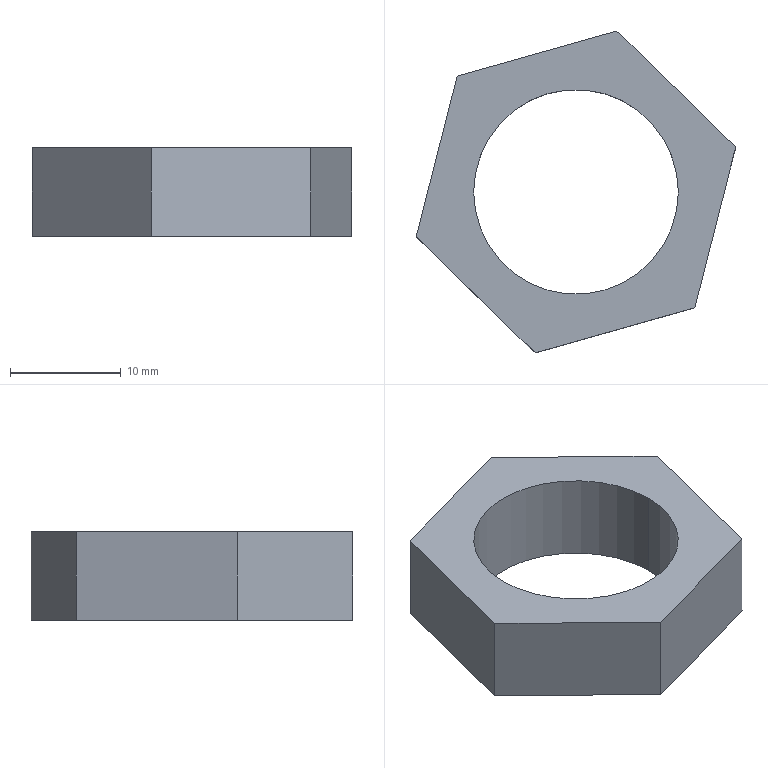Part | STEP file | 1 solid | 10 faces | box 28.896 x 29.097 x 8 mm | volume 2533 mm3 | plane 8 | cylinder 2 | commonest cylinder face diameters 18.5 x2
STEP:
#1=CARTESIAN_POINT('',(0.,0.,0.));
#2=DIRECTION('',(0.,0.,1.));
#3=DIRECTION('',(1.,0.,0.));
#4=AXIS2_PLACEMENT_3D('',#1,#2,#3);
#5=CARTESIAN_POINT('',(9.25,0.,0.));
#6=VERTEX_POINT('',#5);
#7=CARTESIAN_POINT('',(9.25,0.,8.));
#8=VERTEX_POINT('',#7);
#9=CARTESIAN_POINT('',(9.25,0.,0.));
#10=DIRECTION('',(0.,0.,1.));
#11=VECTOR('',#10,1.);
#12=LINE('',#9,#11);
#13=CARTESIAN_POINT('',(0.,0.,0.));
#14=DIRECTION('',(0.,0.,1.));
#15=DIRECTION('',(1.,0.,0.));
#16=AXIS2_PLACEMENT_3D('',#13,#14,#15);
#17=CYLINDRICAL_SURFACE('',#16,9.25);
#18=CARTESIAN_POINT('',(6.283,0.));
#19=DIRECTION('',(0.,1.));
#20=VECTOR('',#19,1.);
#21=LINE('',#18,#20);
#22=(GEOMETRIC_REPRESENTATION_CONTEXT(2)PARAMETRIC_REPRESENTATION_CONTEXT()REPRESENTATION_CONTEXT('',''));
#23=DEFINITIONAL_REPRESENTATION('',(#21),#22);
#24=PCURVE('',#17,#23);
#25=CARTESIAN_POINT('',(0.,0.,0.));
#26=DIRECTION('',(0.,0.,1.));
#27=DIRECTION('',(1.,0.,0.));
#28=AXIS2_PLACEMENT_3D('',#25,#26,#27);
#29=CYLINDRICAL_SURFACE('',#28,9.25);
#30=CARTESIAN_POINT('',(0.,0.));
#31=DIRECTION('',(0.,1.));
#32=VECTOR('',#31,1.);
#33=LINE('',#30,#32);
#34=(GEOMETRIC_REPRESENTATION_CONTEXT(2)PARAMETRIC_REPRESENTATION_CONTEXT()REPRESENTATION_CONTEXT('',''));
#35=DEFINITIONAL_REPRESENTATION('',(#33),#34);
#36=PCURVE('',#29,#35);
#37=SURFACE_CURVE('',#12,(#24,#36),.PCURVE_S1.);
#38=EDGE_CURVE('',#6,#8,#37,.T.);
#39=ORIENTED_EDGE('',*,*,#38,.T.);
#40=CARTESIAN_POINT('',(-9.25,0.,8.));
#41=VERTEX_POINT('',#40);
#42=CARTESIAN_POINT('',(0.,0.,8.));
#43=DIRECTION('',(0.,0.,1.));
#44=DIRECTION('',(1.,0.,0.));
#45=AXIS2_PLACEMENT_3D('',#42,#43,#44);
#46=CIRCLE('',#45,9.25);
#47=CARTESIAN_POINT('',(0.,8.));
#48=DIRECTION('',(1.,0.));
#49=VECTOR('',#48,1.);
#50=LINE('',#47,#49);
#51=(GEOMETRIC_REPRESENTATION_CONTEXT(2)PARAMETRIC_REPRESENTATION_CONTEXT()REPRESENTATION_CONTEXT('',''));
#52=DEFINITIONAL_REPRESENTATION('',(#50),#51);
#53=PCURVE('',#17,#52);
#54=CARTESIAN_POINT('',(-14.622,-14.723,8.));
#55=DIRECTION('',(0.,0.,1.));
#56=DIRECTION('',(1.,0.,0.));
#57=AXIS2_PLACEMENT_3D('',#54,#55,#56);
#58=PLANE('',#57);
#59=CARTESIAN_POINT('',(14.622,14.723));
#60=DIRECTION('',(1.,0.));
#61=AXIS2_PLACEMENT_2D('',#59,#60);
#62=CIRCLE('',#61,9.25);
#63=(GEOMETRIC_REPRESENTATION_CONTEXT(2)PARAMETRIC_REPRESENTATION_CONTEXT()REPRESENTATION_CONTEXT('',''));
#64=DEFINITIONAL_REPRESENTATION('',(#62),#63);
#65=PCURVE('',#58,#64);
#66=SURFACE_CURVE('',#46,(#53,#65),.PCURVE_S1.);
#67=EDGE_CURVE('',#41,#8,#66,.T.);
#68=ORIENTED_EDGE('',*,*,#67,.F.);
#69=CARTESIAN_POINT('',(-9.25,0.,0.));
#70=VERTEX_POINT('',#69);
#71=CARTESIAN_POINT('',(-9.25,0.,0.));
#72=DIRECTION('',(0.,0.,1.));
#73=VECTOR('',#72,1.);
#74=LINE('',#71,#73);
#75=CARTESIAN_POINT('',(3.142,0.));
#76=DIRECTION('',(0.,1.));
#77=VECTOR('',#76,1.);
#78=LINE('',#75,#77);
#79=(GEOMETRIC_REPRESENTATION_CONTEXT(2)PARAMETRIC_REPRESENTATION_CONTEXT()REPRESENTATION_CONTEXT('',''));
#80=DEFINITIONAL_REPRESENTATION('',(#78),#79);
#81=PCURVE('',#17,#80);
#82=CARTESIAN_POINT('',(3.142,0.));
#83=DIRECTION('',(0.,1.));
#84=VECTOR('',#83,1.);
#85=LINE('',#82,#84);
#86=(GEOMETRIC_REPRESENTATION_CONTEXT(2)PARAMETRIC_REPRESENTATION_CONTEXT()REPRESENTATION_CONTEXT('',''));
#87=DEFINITIONAL_REPRESENTATION('',(#85),#86);
#88=PCURVE('',#29,#87);
#89=SURFACE_CURVE('',#74,(#81,#88),.PCURVE_S1.);
#90=EDGE_CURVE('',#70,#41,#89,.T.);
#91=ORIENTED_EDGE('',*,*,#90,.F.);
#92=CARTESIAN_POINT('',(0.,0.,0.));
#93=DIRECTION('',(0.,0.,-1.));
#94=DIRECTION('',(1.,0.,0.));
#95=AXIS2_PLACEMENT_3D('',#92,#93,#94);
#96=CIRCLE('',#95,9.25);
#97=CARTESIAN_POINT('',(6.283,0.));
#98=DIRECTION('',(-1.,0.));
#99=VECTOR('',#98,1.);
#100=LINE('',#97,#99);
#101=(GEOMETRIC_REPRESENTATION_CONTEXT(2)PARAMETRIC_REPRESENTATION_CONTEXT()REPRESENTATION_CONTEXT('',''));
#102=DEFINITIONAL_REPRESENTATION('',(#100),#101);
#103=PCURVE('',#17,#102);
#104=CARTESIAN_POINT('',(-14.622,-14.723,0.));
#105=DIRECTION('',(0.,0.,1.));
#106=DIRECTION('',(1.,0.,0.));
#107=AXIS2_PLACEMENT_3D('',#104,#105,#106);
#108=PLANE('',#107);
#109=CARTESIAN_POINT('',(23.872,14.723));
#110=CARTESIAN_POINT('',(23.872,-1.298));
#111=CARTESIAN_POINT('',(9.997,6.712));
#112=CARTESIAN_POINT('',(-3.878,14.723));
#113=CARTESIAN_POINT('',(9.997,22.734));
#114=CARTESIAN_POINT('',(23.872,30.745));
#115=CARTESIAN_POINT('',(23.872,14.723));
#116=(BOUNDED_CURVE()B_SPLINE_CURVE(2,(#109,#110,#111,#112,#113,#114,#115),.UNSPECIFIED.,.T.,.F.)B_SPLINE_CURVE_WITH_KNOTS((1,2,2,2,2,1),(-2.094,0.,2.094,4.189,6.283,8.378),.UNSPECIFIED.)CURVE()GEOMETRIC_REPRESENTATION_ITEM()RATIONAL_B_SPLINE_CURVE((1.,0.5,1.,0.5,1.,0.5,1.))REPRESENTATION_ITEM(''));
#117=(GEOMETRIC_REPRESENTATION_CONTEXT(2)PARAMETRIC_REPRESENTATION_CONTEXT()REPRESENTATION_CONTEXT('',''));
#118=DEFINITIONAL_REPRESENTATION('',(#116),#117);
#119=PCURVE('',#108,#118);
#120=SURFACE_CURVE('',#96,(#103,#119),.PCURVE_S1.);
#121=EDGE_CURVE('',#6,#70,#120,.T.);
#122=ORIENTED_EDGE('',*,*,#121,.F.);
#123=EDGE_LOOP('',(#39,#68,#91,#122));
#124=FACE_BOUND('',#123,.F.);
#125=ADVANCED_FACE('',(#124),#17,.F.);
#126=CARTESIAN_POINT('',(0.,0.,8.));
#127=DIRECTION('',(0.,0.,1.));
#128=DIRECTION('',(1.,0.,0.));
#129=AXIS2_PLACEMENT_3D('',#126,#127,#128);
#130=CIRCLE('',#129,9.25);
#131=CARTESIAN_POINT('',(0.,8.));
#132=DIRECTION('',(1.,0.));
#133=VECTOR('',#132,1.);
#134=LINE('',#131,#133);
#135=(GEOMETRIC_REPRESENTATION_CONTEXT(2)PARAMETRIC_REPRESENTATION_CONTEXT()REPRESENTATION_CONTEXT('',''));
#136=DEFINITIONAL_REPRESENTATION('',(#134),#135);
#137=PCURVE('',#29,#136);
#138=CARTESIAN_POINT('',(14.622,14.723));
#139=DIRECTION('',(1.,0.));
#140=AXIS2_PLACEMENT_2D('',#138,#139);
#141=CIRCLE('',#140,9.25);
#142=(GEOMETRIC_REPRESENTATION_CONTEXT(2)PARAMETRIC_REPRESENTATION_CONTEXT()REPRESENTATION_CONTEXT('',''));
#143=DEFINITIONAL_REPRESENTATION('',(#141),#142);
#144=PCURVE('',#58,#143);
#145=SURFACE_CURVE('',#130,(#137,#144),.PCURVE_S1.);
#146=EDGE_CURVE('',#8,#41,#145,.T.);
#147=ORIENTED_EDGE('',*,*,#146,.F.);
#148=ORIENTED_EDGE('',*,*,#38,.F.);
#149=CARTESIAN_POINT('',(0.,0.,0.));
#150=DIRECTION('',(0.,0.,-1.));
#151=DIRECTION('',(1.,0.,0.));
#152=AXIS2_PLACEMENT_3D('',#149,#150,#151);
#153=CIRCLE('',#152,9.25);
#154=CARTESIAN_POINT('',(6.283,0.));
#155=DIRECTION('',(-1.,0.));
#156=VECTOR('',#155,1.);
#157=LINE('',#154,#156);
#158=(GEOMETRIC_REPRESENTATION_CONTEXT(2)PARAMETRIC_REPRESENTATION_CONTEXT()REPRESENTATION_CONTEXT('',''));
#159=DEFINITIONAL_REPRESENTATION('',(#157),#158);
#160=PCURVE('',#29,#159);
#161=CARTESIAN_POINT('',(23.872,14.723));
#162=CARTESIAN_POINT('',(23.872,-1.298));
#163=CARTESIAN_POINT('',(9.997,6.712));
#164=CARTESIAN_POINT('',(-3.878,14.723));
#165=CARTESIAN_POINT('',(9.997,22.734));
#166=CARTESIAN_POINT('',(23.872,30.745));
#167=CARTESIAN_POINT('',(23.872,14.723));
#168=(BOUNDED_CURVE()B_SPLINE_CURVE(2,(#161,#162,#163,#164,#165,#166,#167),.UNSPECIFIED.,.T.,.F.)B_SPLINE_CURVE_WITH_KNOTS((1,2,2,2,2,1),(-2.094,0.,2.094,4.189,6.283,8.378),.UNSPECIFIED.)CURVE()GEOMETRIC_REPRESENTATION_ITEM()RATIONAL_B_SPLINE_CURVE((1.,0.5,1.,0.5,1.,0.5,1.))REPRESENTATION_ITEM(''));
#169=(GEOMETRIC_REPRESENTATION_CONTEXT(2)PARAMETRIC_REPRESENTATION_CONTEXT()REPRESENTATION_CONTEXT('',''));
#170=DEFINITIONAL_REPRESENTATION('',(#168),#169);
#171=PCURVE('',#108,#170);
#172=SURFACE_CURVE('',#153,(#160,#171),.PCURVE_S1.);
#173=EDGE_CURVE('',#70,#6,#172,.T.);
#174=ORIENTED_EDGE('',*,*,#173,.F.);
#175=ORIENTED_EDGE('',*,*,#90,.T.);
#176=EDGE_LOOP('',(#147,#148,#174,#175));
#177=FACE_BOUND('',#176,.F.);
#178=ADVANCED_FACE('',(#177),#29,.F.);
#179=ORIENTED_EDGE('',*,*,#146,.F.);
#180=ORIENTED_EDGE('',*,*,#67,.F.);
#181=EDGE_LOOP('',(#179,#180));
#182=FACE_BOUND('',#181,.T.);
#183=CARTESIAN_POINT('',(-10.751,10.476,8.));
#184=VERTEX_POINT('',#183);
#185=CARTESIAN_POINT('',(-14.448,-4.072,8.));
#186=VERTEX_POINT('',#185);
#187=CARTESIAN_POINT('',(-10.751,10.476,8.));
#188=DIRECTION('',(-0.2463,-0.9692,0.));
#189=VECTOR('',#188,1.);
#190=LINE('',#187,#189);
#191=CARTESIAN_POINT('',(3.871,25.2));
#192=DIRECTION('',(-0.2463,-0.9692));
#193=VECTOR('',#192,1.);
#194=LINE('',#191,#193);
#195=(GEOMETRIC_REPRESENTATION_CONTEXT(2)PARAMETRIC_REPRESENTATION_CONTEXT()REPRESENTATION_CONTEXT('',''));
#196=DEFINITIONAL_REPRESENTATION('',(#194),#195);
#197=PCURVE('',#58,#196);
#198=CARTESIAN_POINT('',(-14.448,-4.072,0.));
#199=DIRECTION('',(0.9692,-0.2463,0.));
#200=DIRECTION('',(0.2463,0.9692,0.));
#201=AXIS2_PLACEMENT_3D('',#198,#199,#200);
#202=PLANE('',#201);
#203=CARTESIAN_POINT('',(15.011,8.));
#204=DIRECTION('',(-1.,0.));
#205=VECTOR('',#204,1.);
#206=LINE('',#203,#205);
#207=(GEOMETRIC_REPRESENTATION_CONTEXT(2)PARAMETRIC_REPRESENTATION_CONTEXT()REPRESENTATION_CONTEXT('',''));
#208=DEFINITIONAL_REPRESENTATION('',(#206),#207);
#209=PCURVE('',#202,#208);
#210=SURFACE_CURVE('',#190,(#197,#209),.PCURVE_S1.);
#211=EDGE_CURVE('',#184,#186,#210,.T.);
#212=ORIENTED_EDGE('',*,*,#211,.T.);
#213=CARTESIAN_POINT('',(-3.698,-14.549,8.));
#214=VERTEX_POINT('',#213);
#215=CARTESIAN_POINT('',(-14.448,-4.072,8.));
#216=DIRECTION('',(0.7162,-0.6979,0.));
#217=VECTOR('',#216,1.);
#218=LINE('',#215,#217);
#219=CARTESIAN_POINT('',(0.1734,10.651));
#220=DIRECTION('',(0.7162,-0.6979));
#221=VECTOR('',#220,1.);
#222=LINE('',#219,#221);
#223=(GEOMETRIC_REPRESENTATION_CONTEXT(2)PARAMETRIC_REPRESENTATION_CONTEXT()REPRESENTATION_CONTEXT('',''));
#224=DEFINITIONAL_REPRESENTATION('',(#222),#223);
#225=PCURVE('',#58,#224);
#226=CARTESIAN_POINT('',(-3.698,-14.549,0.));
#227=DIRECTION('',(0.6979,0.7162,0.));
#228=DIRECTION('',(-0.7162,0.6979,0.));
#229=AXIS2_PLACEMENT_3D('',#226,#227,#228);
#230=PLANE('',#229);
#231=CARTESIAN_POINT('',(15.011,8.));
#232=DIRECTION('',(-1.,0.));
#233=VECTOR('',#232,1.);
#234=LINE('',#231,#233);
#235=(GEOMETRIC_REPRESENTATION_CONTEXT(2)PARAMETRIC_REPRESENTATION_CONTEXT()REPRESENTATION_CONTEXT('',''));
#236=DEFINITIONAL_REPRESENTATION('',(#234),#235);
#237=PCURVE('',#230,#236);
#238=SURFACE_CURVE('',#218,(#225,#237),.PCURVE_S1.);
#239=EDGE_CURVE('',#186,#214,#238,.T.);
#240=ORIENTED_EDGE('',*,*,#239,.T.);
#241=CARTESIAN_POINT('',(10.751,-10.476,8.));
#242=VERTEX_POINT('',#241);
#243=CARTESIAN_POINT('',(-3.698,-14.549,8.));
#244=DIRECTION('',(0.9625,0.2713,0.));
#245=VECTOR('',#244,1.);
#246=LINE('',#243,#245);
#247=CARTESIAN_POINT('',(10.924,0.1746));
#248=DIRECTION('',(0.9625,0.2713));
#249=VECTOR('',#248,1.);
#250=LINE('',#247,#249);
#251=(GEOMETRIC_REPRESENTATION_CONTEXT(2)PARAMETRIC_REPRESENTATION_CONTEXT()REPRESENTATION_CONTEXT('',''));
#252=DEFINITIONAL_REPRESENTATION('',(#250),#251);
#253=PCURVE('',#58,#252);
#254=CARTESIAN_POINT('',(10.751,-10.476,0.));
#255=DIRECTION('',(-0.2713,0.9625,0.));
#256=DIRECTION('',(-0.9625,-0.2713,0.));
#257=AXIS2_PLACEMENT_3D('',#254,#255,#256);
#258=PLANE('',#257);
#259=CARTESIAN_POINT('',(15.011,8.));
#260=DIRECTION('',(-1.,0.));
#261=VECTOR('',#260,1.);
#262=LINE('',#259,#261);
#263=(GEOMETRIC_REPRESENTATION_CONTEXT(2)PARAMETRIC_REPRESENTATION_CONTEXT()REPRESENTATION_CONTEXT('',''));
#264=DEFINITIONAL_REPRESENTATION('',(#262),#263);
#265=PCURVE('',#258,#264);
#266=SURFACE_CURVE('',#246,(#253,#265),.PCURVE_S1.);
#267=EDGE_CURVE('',#214,#242,#266,.T.);
#268=ORIENTED_EDGE('',*,*,#267,.T.);
#269=CARTESIAN_POINT('',(14.448,4.072,8.));
#270=VERTEX_POINT('',#269);
#271=CARTESIAN_POINT('',(10.751,-10.476,8.));
#272=DIRECTION('',(0.2463,0.9692,0.));
#273=VECTOR('',#272,1.);
#274=LINE('',#271,#273);
#275=CARTESIAN_POINT('',(25.372,4.247));
#276=DIRECTION('',(0.2463,0.9692));
#277=VECTOR('',#276,1.);
#278=LINE('',#275,#277);
#279=(GEOMETRIC_REPRESENTATION_CONTEXT(2)PARAMETRIC_REPRESENTATION_CONTEXT()REPRESENTATION_CONTEXT('',''));
#280=DEFINITIONAL_REPRESENTATION('',(#278),#279);
#281=PCURVE('',#58,#280);
#282=CARTESIAN_POINT('',(14.448,4.072,0.));
#283=DIRECTION('',(-0.9692,0.2463,0.));
#284=DIRECTION('',(-0.2463,-0.9692,0.));
#285=AXIS2_PLACEMENT_3D('',#282,#283,#284);
#286=PLANE('',#285);
#287=CARTESIAN_POINT('',(15.011,8.));
#288=DIRECTION('',(-1.,0.));
#289=VECTOR('',#288,1.);
#290=LINE('',#287,#289);
#291=(GEOMETRIC_REPRESENTATION_CONTEXT(2)PARAMETRIC_REPRESENTATION_CONTEXT()REPRESENTATION_CONTEXT('',''));
#292=DEFINITIONAL_REPRESENTATION('',(#290),#291);
#293=PCURVE('',#286,#292);
#294=SURFACE_CURVE('',#274,(#281,#293),.PCURVE_S1.);
#295=EDGE_CURVE('',#242,#270,#294,.T.);
#296=ORIENTED_EDGE('',*,*,#295,.T.);
#297=CARTESIAN_POINT('',(3.698,14.549,8.));
#298=VERTEX_POINT('',#297);
#299=CARTESIAN_POINT('',(14.448,4.072,8.));
#300=DIRECTION('',(-0.7162,0.6979,0.));
#301=VECTOR('',#300,1.);
#302=LINE('',#299,#301);
#303=CARTESIAN_POINT('',(29.07,18.795));
#304=DIRECTION('',(-0.7162,0.6979));
#305=VECTOR('',#304,1.);
#306=LINE('',#303,#305);
#307=(GEOMETRIC_REPRESENTATION_CONTEXT(2)PARAMETRIC_REPRESENTATION_CONTEXT()REPRESENTATION_CONTEXT('',''));
#308=DEFINITIONAL_REPRESENTATION('',(#306),#307);
#309=PCURVE('',#58,#308);
#310=CARTESIAN_POINT('',(3.698,14.549,0.));
#311=DIRECTION('',(-0.6979,-0.7162,0.));
#312=DIRECTION('',(0.7162,-0.6979,0.));
#313=AXIS2_PLACEMENT_3D('',#310,#311,#312);
#314=PLANE('',#313);
#315=CARTESIAN_POINT('',(15.011,8.));
#316=DIRECTION('',(-1.,0.));
#317=VECTOR('',#316,1.);
#318=LINE('',#315,#317);
#319=(GEOMETRIC_REPRESENTATION_CONTEXT(2)PARAMETRIC_REPRESENTATION_CONTEXT()REPRESENTATION_CONTEXT('',''));
#320=DEFINITIONAL_REPRESENTATION('',(#318),#319);
#321=PCURVE('',#314,#320);
#322=SURFACE_CURVE('',#302,(#309,#321),.PCURVE_S1.);
#323=EDGE_CURVE('',#270,#298,#322,.T.);
#324=ORIENTED_EDGE('',*,*,#323,.T.);
#325=CARTESIAN_POINT('',(3.698,14.549,8.));
#326=DIRECTION('',(-0.9625,-0.2713,0.));
#327=VECTOR('',#326,1.);
#328=LINE('',#325,#327);
#329=CARTESIAN_POINT('',(18.319,29.272));
#330=DIRECTION('',(-0.9625,-0.2713));
#331=VECTOR('',#330,1.);
#332=LINE('',#329,#331);
#333=(GEOMETRIC_REPRESENTATION_CONTEXT(2)PARAMETRIC_REPRESENTATION_CONTEXT()REPRESENTATION_CONTEXT('',''));
#334=DEFINITIONAL_REPRESENTATION('',(#332),#333);
#335=PCURVE('',#58,#334);
#336=CARTESIAN_POINT('',(-10.751,10.476,0.));
#337=DIRECTION('',(0.2713,-0.9625,0.));
#338=DIRECTION('',(0.9625,0.2713,0.));
#339=AXIS2_PLACEMENT_3D('',#336,#337,#338);
#340=PLANE('',#339);
#341=CARTESIAN_POINT('',(15.011,8.));
#342=DIRECTION('',(-1.,0.));
#343=VECTOR('',#342,1.);
#344=LINE('',#341,#343);
#345=(GEOMETRIC_REPRESENTATION_CONTEXT(2)PARAMETRIC_REPRESENTATION_CONTEXT()REPRESENTATION_CONTEXT('',''));
#346=DEFINITIONAL_REPRESENTATION('',(#344),#345);
#347=PCURVE('',#340,#346);
#348=SURFACE_CURVE('',#328,(#335,#347),.PCURVE_S1.);
#349=EDGE_CURVE('',#298,#184,#348,.T.);
#350=ORIENTED_EDGE('',*,*,#349,.T.);
#351=EDGE_LOOP('',(#212,#240,#268,#296,#324,#350));
#352=FACE_BOUND('',#351,.T.);
#353=ADVANCED_FACE('',(#182,#352),#58,.T.);
#354=ORIENTED_EDGE('',*,*,#121,.F.);
#355=ORIENTED_EDGE('',*,*,#173,.F.);
#356=EDGE_LOOP('',(#354,#355));
#357=FACE_BOUND('',#356,.T.);
#358=CARTESIAN_POINT('',(-14.448,-4.072,0.));
#359=VERTEX_POINT('',#358);
#360=CARTESIAN_POINT('',(-3.698,-14.549,0.));
#361=VERTEX_POINT('',#360);
#362=CARTESIAN_POINT('',(-3.698,-14.549,0.));
#363=DIRECTION('',(0.7162,-0.6979,0.));
#364=VECTOR('',#363,1.);
#365=LINE('',#362,#364);
#366=CARTESIAN_POINT('',(10.924,0.1746));
#367=DIRECTION('',(0.7162,-0.6979));
#368=VECTOR('',#367,1.);
#369=LINE('',#366,#368);
#370=(GEOMETRIC_REPRESENTATION_CONTEXT(2)PARAMETRIC_REPRESENTATION_CONTEXT()REPRESENTATION_CONTEXT('',''));
#371=DEFINITIONAL_REPRESENTATION('',(#369),#370);
#372=PCURVE('',#108,#371);
#373=CARTESIAN_POINT('',(0.,0.));
#374=DIRECTION('',(-1.,0.));
#375=VECTOR('',#374,1.);
#376=LINE('',#373,#375);
#377=(GEOMETRIC_REPRESENTATION_CONTEXT(2)PARAMETRIC_REPRESENTATION_CONTEXT()REPRESENTATION_CONTEXT('',''));
#378=DEFINITIONAL_REPRESENTATION('',(#376),#377);
#379=PCURVE('',#230,#378);
#380=SURFACE_CURVE('',#365,(#372,#379),.PCURVE_S1.);
#381=EDGE_CURVE('',#359,#361,#380,.T.);
#382=ORIENTED_EDGE('',*,*,#381,.F.);
#383=CARTESIAN_POINT('',(-10.751,10.476,0.));
#384=VERTEX_POINT('',#383);
#385=CARTESIAN_POINT('',(-14.448,-4.072,0.));
#386=DIRECTION('',(-0.2463,-0.9692,0.));
#387=VECTOR('',#386,1.);
#388=LINE('',#385,#387);
#389=CARTESIAN_POINT('',(0.1734,10.651));
#390=DIRECTION('',(-0.2463,-0.9692));
#391=VECTOR('',#390,1.);
#392=LINE('',#389,#391);
#393=(GEOMETRIC_REPRESENTATION_CONTEXT(2)PARAMETRIC_REPRESENTATION_CONTEXT()REPRESENTATION_CONTEXT('',''));
#394=DEFINITIONAL_REPRESENTATION('',(#392),#393);
#395=PCURVE('',#108,#394);
#396=CARTESIAN_POINT('',(0.,0.));
#397=DIRECTION('',(-1.,0.));
#398=VECTOR('',#397,1.);
#399=LINE('',#396,#398);
#400=(GEOMETRIC_REPRESENTATION_CONTEXT(2)PARAMETRIC_REPRESENTATION_CONTEXT()REPRESENTATION_CONTEXT('',''));
#401=DEFINITIONAL_REPRESENTATION('',(#399),#400);
#402=PCURVE('',#202,#401);
#403=SURFACE_CURVE('',#388,(#395,#402),.PCURVE_S1.);
#404=EDGE_CURVE('',#384,#359,#403,.T.);
#405=ORIENTED_EDGE('',*,*,#404,.F.);
#406=CARTESIAN_POINT('',(3.698,14.549,0.));
#407=VERTEX_POINT('',#406);
#408=CARTESIAN_POINT('',(-10.751,10.476,0.));
#409=DIRECTION('',(-0.9625,-0.2713,0.));
#410=VECTOR('',#409,1.);
#411=LINE('',#408,#410);
#412=CARTESIAN_POINT('',(3.871,25.2));
#413=DIRECTION('',(-0.9625,-0.2713));
#414=VECTOR('',#413,1.);
#415=LINE('',#412,#414);
#416=(GEOMETRIC_REPRESENTATION_CONTEXT(2)PARAMETRIC_REPRESENTATION_CONTEXT()REPRESENTATION_CONTEXT('',''));
#417=DEFINITIONAL_REPRESENTATION('',(#415),#416);
#418=PCURVE('',#108,#417);
#419=CARTESIAN_POINT('',(0.,0.));
#420=DIRECTION('',(-1.,0.));
#421=VECTOR('',#420,1.);
#422=LINE('',#419,#421);
#423=(GEOMETRIC_REPRESENTATION_CONTEXT(2)PARAMETRIC_REPRESENTATION_CONTEXT()REPRESENTATION_CONTEXT('',''));
#424=DEFINITIONAL_REPRESENTATION('',(#422),#423);
#425=PCURVE('',#340,#424);
#426=SURFACE_CURVE('',#411,(#418,#425),.PCURVE_S1.);
#427=EDGE_CURVE('',#407,#384,#426,.T.);
#428=ORIENTED_EDGE('',*,*,#427,.F.);
#429=CARTESIAN_POINT('',(14.448,4.072,0.));
#430=VERTEX_POINT('',#429);
#431=CARTESIAN_POINT('',(3.698,14.549,0.));
#432=DIRECTION('',(-0.7162,0.6979,0.));
#433=VECTOR('',#432,1.);
#434=LINE('',#431,#433);
#435=CARTESIAN_POINT('',(18.319,29.272));
#436=DIRECTION('',(-0.7162,0.6979));
#437=VECTOR('',#436,1.);
#438=LINE('',#435,#437);
#439=(GEOMETRIC_REPRESENTATION_CONTEXT(2)PARAMETRIC_REPRESENTATION_CONTEXT()REPRESENTATION_CONTEXT('',''));
#440=DEFINITIONAL_REPRESENTATION('',(#438),#439);
#441=PCURVE('',#108,#440);
#442=CARTESIAN_POINT('',(0.,0.));
#443=DIRECTION('',(-1.,0.));
#444=VECTOR('',#443,1.);
#445=LINE('',#442,#444);
#446=(GEOMETRIC_REPRESENTATION_CONTEXT(2)PARAMETRIC_REPRESENTATION_CONTEXT()REPRESENTATION_CONTEXT('',''));
#447=DEFINITIONAL_REPRESENTATION('',(#445),#446);
#448=PCURVE('',#314,#447);
#449=SURFACE_CURVE('',#434,(#441,#448),.PCURVE_S1.);
#450=EDGE_CURVE('',#430,#407,#449,.T.);
#451=ORIENTED_EDGE('',*,*,#450,.F.);
#452=CARTESIAN_POINT('',(10.751,-10.476,0.));
#453=VERTEX_POINT('',#452);
#454=CARTESIAN_POINT('',(14.448,4.072,0.));
#455=DIRECTION('',(0.2463,0.9692,0.));
#456=VECTOR('',#455,1.);
#457=LINE('',#454,#456);
#458=CARTESIAN_POINT('',(29.07,18.795));
#459=DIRECTION('',(0.2463,0.9692));
#460=VECTOR('',#459,1.);
#461=LINE('',#458,#460);
#462=(GEOMETRIC_REPRESENTATION_CONTEXT(2)PARAMETRIC_REPRESENTATION_CONTEXT()REPRESENTATION_CONTEXT('',''));
#463=DEFINITIONAL_REPRESENTATION('',(#461),#462);
#464=PCURVE('',#108,#463);
#465=CARTESIAN_POINT('',(0.,0.));
#466=DIRECTION('',(-1.,0.));
#467=VECTOR('',#466,1.);
#468=LINE('',#465,#467);
#469=(GEOMETRIC_REPRESENTATION_CONTEXT(2)PARAMETRIC_REPRESENTATION_CONTEXT()REPRESENTATION_CONTEXT('',''));
#470=DEFINITIONAL_REPRESENTATION('',(#468),#469);
#471=PCURVE('',#286,#470);
#472=SURFACE_CURVE('',#457,(#464,#471),.PCURVE_S1.);
#473=EDGE_CURVE('',#453,#430,#472,.T.);
#474=ORIENTED_EDGE('',*,*,#473,.F.);
#475=CARTESIAN_POINT('',(10.751,-10.476,0.));
#476=DIRECTION('',(0.9625,0.2713,0.));
#477=VECTOR('',#476,1.);
#478=LINE('',#475,#477);
#479=CARTESIAN_POINT('',(25.372,4.247));
#480=DIRECTION('',(0.9625,0.2713));
#481=VECTOR('',#480,1.);
#482=LINE('',#479,#481);
#483=(GEOMETRIC_REPRESENTATION_CONTEXT(2)PARAMETRIC_REPRESENTATION_CONTEXT()REPRESENTATION_CONTEXT('',''));
#484=DEFINITIONAL_REPRESENTATION('',(#482),#483);
#485=PCURVE('',#108,#484);
#486=CARTESIAN_POINT('',(0.,0.));
#487=DIRECTION('',(-1.,0.));
#488=VECTOR('',#487,1.);
#489=LINE('',#486,#488);
#490=(GEOMETRIC_REPRESENTATION_CONTEXT(2)PARAMETRIC_REPRESENTATION_CONTEXT()REPRESENTATION_CONTEXT('',''));
#491=DEFINITIONAL_REPRESENTATION('',(#489),#490);
#492=PCURVE('',#258,#491);
#493=SURFACE_CURVE('',#478,(#485,#492),.PCURVE_S1.);
#494=EDGE_CURVE('',#361,#453,#493,.T.);
#495=ORIENTED_EDGE('',*,*,#494,.F.);
#496=EDGE_LOOP('',(#382,#405,#428,#451,#474,#495));
#497=FACE_BOUND('',#496,.T.);
#498=ADVANCED_FACE('',(#357,#497),#108,.F.);
#499=CARTESIAN_POINT('',(-3.698,-14.549,4.));
#500=DIRECTION('',(0.,0.,-1.));
#501=VECTOR('',#500,1.);
#502=LINE('',#499,#501);
#503=CARTESIAN_POINT('',(0.,4.));
#504=DIRECTION('',(0.,-1.));
#505=VECTOR('',#504,1.);
#506=LINE('',#503,#505);
#507=(GEOMETRIC_REPRESENTATION_CONTEXT(2)PARAMETRIC_REPRESENTATION_CONTEXT()REPRESENTATION_CONTEXT('',''));
#508=DEFINITIONAL_REPRESENTATION('',(#506),#507);
#509=PCURVE('',#230,#508);
#510=CARTESIAN_POINT('',(15.011,4.));
#511=DIRECTION('',(0.,-1.));
#512=VECTOR('',#511,1.);
#513=LINE('',#510,#512);
#514=(GEOMETRIC_REPRESENTATION_CONTEXT(2)PARAMETRIC_REPRESENTATION_CONTEXT()REPRESENTATION_CONTEXT('',''));
#515=DEFINITIONAL_REPRESENTATION('',(#513),#514);
#516=PCURVE('',#258,#515);
#517=SURFACE_CURVE('',#502,(#509,#516),.PCURVE_S1.);
#518=EDGE_CURVE('',#214,#361,#517,.T.);
#519=ORIENTED_EDGE('',*,*,#518,.F.);
#520=ORIENTED_EDGE('',*,*,#239,.F.);
#521=CARTESIAN_POINT('',(-14.448,-4.072,4.));
#522=DIRECTION('',(0.,0.,1.));
#523=VECTOR('',#522,1.);
#524=LINE('',#521,#523);
#525=CARTESIAN_POINT('',(15.011,4.));
#526=DIRECTION('',(0.,1.));
#527=VECTOR('',#526,1.);
#528=LINE('',#525,#527);
#529=(GEOMETRIC_REPRESENTATION_CONTEXT(2)PARAMETRIC_REPRESENTATION_CONTEXT()REPRESENTATION_CONTEXT('',''));
#530=DEFINITIONAL_REPRESENTATION('',(#528),#529);
#531=PCURVE('',#230,#530);
#532=CARTESIAN_POINT('',(0.,4.));
#533=DIRECTION('',(0.,1.));
#534=VECTOR('',#533,1.);
#535=LINE('',#532,#534);
#536=(GEOMETRIC_REPRESENTATION_CONTEXT(2)PARAMETRIC_REPRESENTATION_CONTEXT()REPRESENTATION_CONTEXT('',''));
#537=DEFINITIONAL_REPRESENTATION('',(#535),#536);
#538=PCURVE('',#202,#537);
#539=SURFACE_CURVE('',#524,(#531,#538),.PCURVE_S1.);
#540=EDGE_CURVE('',#359,#186,#539,.T.);
#541=ORIENTED_EDGE('',*,*,#540,.F.);
#542=ORIENTED_EDGE('',*,*,#381,.T.);
#543=EDGE_LOOP('',(#519,#520,#541,#542));
#544=FACE_BOUND('',#543,.T.);
#545=ADVANCED_FACE('',(#544),#230,.F.);
#546=ORIENTED_EDGE('',*,*,#540,.T.);
#547=ORIENTED_EDGE('',*,*,#211,.F.);
#548=CARTESIAN_POINT('',(-10.751,10.476,4.));
#549=DIRECTION('',(0.,0.,1.));
#550=VECTOR('',#549,1.);
#551=LINE('',#548,#550);
#552=CARTESIAN_POINT('',(15.011,4.));
#553=DIRECTION('',(0.,1.));
#554=VECTOR('',#553,1.);
#555=LINE('',#552,#554);
#556=(GEOMETRIC_REPRESENTATION_CONTEXT(2)PARAMETRIC_REPRESENTATION_CONTEXT()REPRESENTATION_CONTEXT('',''));
#557=DEFINITIONAL_REPRESENTATION('',(#555),#556);
#558=PCURVE('',#202,#557);
#559=CARTESIAN_POINT('',(0.,4.));
#560=DIRECTION('',(0.,1.));
#561=VECTOR('',#560,1.);
#562=LINE('',#559,#561);
#563=(GEOMETRIC_REPRESENTATION_CONTEXT(2)PARAMETRIC_REPRESENTATION_CONTEXT()REPRESENTATION_CONTEXT('',''));
#564=DEFINITIONAL_REPRESENTATION('',(#562),#563);
#565=PCURVE('',#340,#564);
#566=SURFACE_CURVE('',#551,(#558,#565),.PCURVE_S1.);
#567=EDGE_CURVE('',#384,#184,#566,.T.);
#568=ORIENTED_EDGE('',*,*,#567,.F.);
#569=ORIENTED_EDGE('',*,*,#404,.T.);
#570=EDGE_LOOP('',(#546,#547,#568,#569));
#571=FACE_BOUND('',#570,.T.);
#572=ADVANCED_FACE('',(#571),#202,.F.);
#573=ORIENTED_EDGE('',*,*,#567,.T.);
#574=ORIENTED_EDGE('',*,*,#349,.F.);
#575=CARTESIAN_POINT('',(3.698,14.549,4.));
#576=DIRECTION('',(0.,0.,1.));
#577=VECTOR('',#576,1.);
#578=LINE('',#575,#577);
#579=CARTESIAN_POINT('',(15.011,4.));
#580=DIRECTION('',(0.,1.));
#581=VECTOR('',#580,1.);
#582=LINE('',#579,#581);
#583=(GEOMETRIC_REPRESENTATION_CONTEXT(2)PARAMETRIC_REPRESENTATION_CONTEXT()REPRESENTATION_CONTEXT('',''));
#584=DEFINITIONAL_REPRESENTATION('',(#582),#583);
#585=PCURVE('',#340,#584);
#586=CARTESIAN_POINT('',(0.,4.));
#587=DIRECTION('',(0.,1.));
#588=VECTOR('',#587,1.);
#589=LINE('',#586,#588);
#590=(GEOMETRIC_REPRESENTATION_CONTEXT(2)PARAMETRIC_REPRESENTATION_CONTEXT()REPRESENTATION_CONTEXT('',''));
#591=DEFINITIONAL_REPRESENTATION('',(#589),#590);
#592=PCURVE('',#314,#591);
#593=SURFACE_CURVE('',#578,(#585,#592),.PCURVE_S1.);
#594=EDGE_CURVE('',#407,#298,#593,.T.);
#595=ORIENTED_EDGE('',*,*,#594,.F.);
#596=ORIENTED_EDGE('',*,*,#427,.T.);
#597=EDGE_LOOP('',(#573,#574,#595,#596));
#598=FACE_BOUND('',#597,.T.);
#599=ADVANCED_FACE('',(#598),#340,.F.);
#600=ORIENTED_EDGE('',*,*,#594,.T.);
#601=ORIENTED_EDGE('',*,*,#323,.F.);
#602=CARTESIAN_POINT('',(14.448,4.072,4.));
#603=DIRECTION('',(0.,0.,1.));
#604=VECTOR('',#603,1.);
#605=LINE('',#602,#604);
#606=CARTESIAN_POINT('',(15.011,4.));
#607=DIRECTION('',(0.,1.));
#608=VECTOR('',#607,1.);
#609=LINE('',#606,#608);
#610=(GEOMETRIC_REPRESENTATION_CONTEXT(2)PARAMETRIC_REPRESENTATION_CONTEXT()REPRESENTATION_CONTEXT('',''));
#611=DEFINITIONAL_REPRESENTATION('',(#609),#610);
#612=PCURVE('',#314,#611);
#613=CARTESIAN_POINT('',(0.,4.));
#614=DIRECTION('',(0.,1.));
#615=VECTOR('',#614,1.);
#616=LINE('',#613,#615);
#617=(GEOMETRIC_REPRESENTATION_CONTEXT(2)PARAMETRIC_REPRESENTATION_CONTEXT()REPRESENTATION_CONTEXT('',''));
#618=DEFINITIONAL_REPRESENTATION('',(#616),#617);
#619=PCURVE('',#286,#618);
#620=SURFACE_CURVE('',#605,(#612,#619),.PCURVE_S1.);
#621=EDGE_CURVE('',#430,#270,#620,.T.);
#622=ORIENTED_EDGE('',*,*,#621,.F.);
#623=ORIENTED_EDGE('',*,*,#450,.T.);
#624=EDGE_LOOP('',(#600,#601,#622,#623));
#625=FACE_BOUND('',#624,.T.);
#626=ADVANCED_FACE('',(#625),#314,.F.);
#627=ORIENTED_EDGE('',*,*,#621,.T.);
#628=ORIENTED_EDGE('',*,*,#295,.F.);
#629=CARTESIAN_POINT('',(10.751,-10.476,4.));
#630=DIRECTION('',(0.,0.,1.));
#631=VECTOR('',#630,1.);
#632=LINE('',#629,#631);
#633=CARTESIAN_POINT('',(15.011,4.));
#634=DIRECTION('',(0.,1.));
#635=VECTOR('',#634,1.);
#636=LINE('',#633,#635);
#637=(GEOMETRIC_REPRESENTATION_CONTEXT(2)PARAMETRIC_REPRESENTATION_CONTEXT()REPRESENTATION_CONTEXT('',''));
#638=DEFINITIONAL_REPRESENTATION('',(#636),#637);
#639=PCURVE('',#286,#638);
#640=CARTESIAN_POINT('',(0.,4.));
#641=DIRECTION('',(0.,1.));
#642=VECTOR('',#641,1.);
#643=LINE('',#640,#642);
#644=(GEOMETRIC_REPRESENTATION_CONTEXT(2)PARAMETRIC_REPRESENTATION_CONTEXT()REPRESENTATION_CONTEXT('',''));
#645=DEFINITIONAL_REPRESENTATION('',(#643),#644);
#646=PCURVE('',#258,#645);
#647=SURFACE_CURVE('',#632,(#639,#646),.PCURVE_S1.);
#648=EDGE_CURVE('',#453,#242,#647,.T.);
#649=ORIENTED_EDGE('',*,*,#648,.F.);
#650=ORIENTED_EDGE('',*,*,#473,.T.);
#651=EDGE_LOOP('',(#627,#628,#649,#650));
#652=FACE_BOUND('',#651,.T.);
#653=ADVANCED_FACE('',(#652),#286,.F.);
#654=ORIENTED_EDGE('',*,*,#648,.T.);
#655=ORIENTED_EDGE('',*,*,#267,.F.);
#656=ORIENTED_EDGE('',*,*,#518,.T.);
#657=ORIENTED_EDGE('',*,*,#494,.T.);
#658=EDGE_LOOP('',(#654,#655,#656,#657));
#659=FACE_BOUND('',#658,.T.);
#660=ADVANCED_FACE('',(#659),#258,.F.);
#661=CLOSED_SHELL('',(#125,#178,#353,#498,#545,#572,#599,#626,#653,#660));
#662=MANIFOLD_SOLID_BREP('',#661);
#663=(LENGTH_UNIT()NAMED_UNIT(*)SI_UNIT(.MILLI.,.METRE.));
#664=UNCERTAINTY_MEASURE_WITH_UNIT(LENGTH_MEASURE(0.0000001),#663,'','');
#665=(NAMED_UNIT(*)PLANE_ANGLE_UNIT()SI_UNIT($,.RADIAN.));
#666=(NAMED_UNIT(*)SI_UNIT($,.STERADIAN.)SOLID_ANGLE_UNIT());
#667=(GEOMETRIC_REPRESENTATION_CONTEXT(3)GLOBAL_UNCERTAINTY_ASSIGNED_CONTEXT((#664))GLOBAL_UNIT_ASSIGNED_CONTEXT((#663,#665,#666))REPRESENTATION_CONTEXT('',''));
#668=ADVANCED_BREP_SHAPE_REPRESENTATION('',(#4,#662),#667);